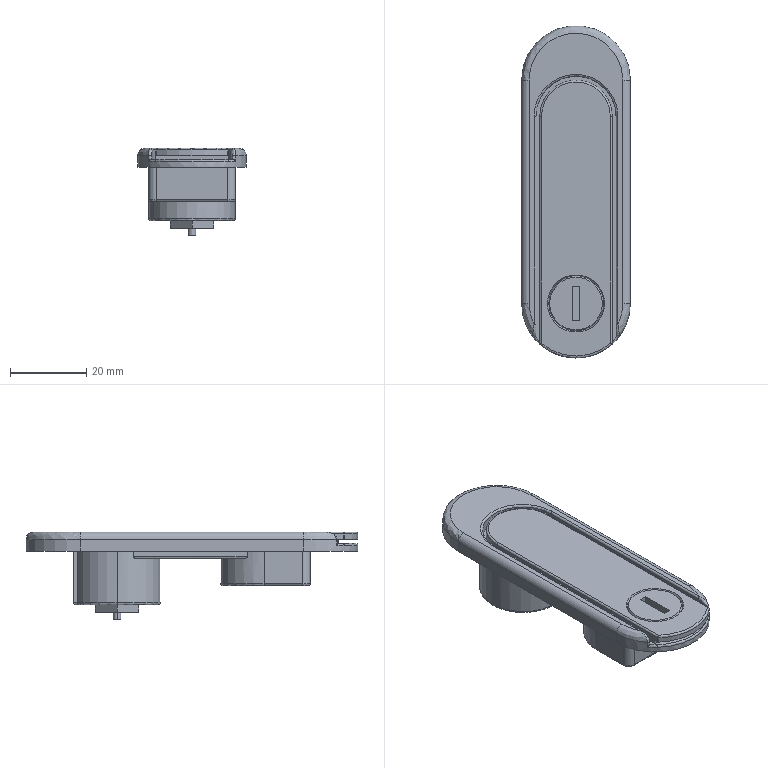Part | STEP file | 11-GYAB403-1.-23011111 | 1 solid | 92 faces | box 28.5 x 87 x 23 mm | volume 21760 mm3 | plane 36 | cylinder 32 | spline 20 | cone 4 | commonest cylinder face diameters 1 x17 4 x4 22.7 x3 28.5 x3 1.994 x2 19 x1